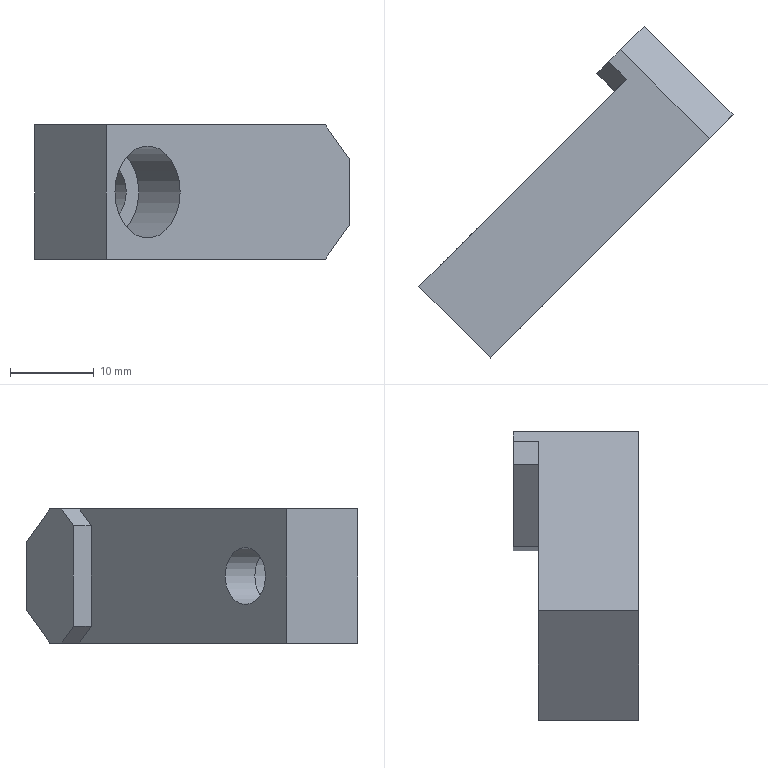Part | STEP file | gslz 2016.10.28-13_id1390_x_t | 1 solid | 15 faces | box 37.477 x 39.598 x 16 mm | volume 7157 mm3 | plane 13 | cylinder 2 | commonest cylinder face diameters 6.8 x1 11 x1
STEP:
#1=CARTESIAN_POINT('',(0.,0.,0.));
#2=DIRECTION('',(0.,0.,1.));
#3=DIRECTION('',(1.,0.,0.));
#4=AXIS2_PLACEMENT_3D('',#1,#2,#3);
#5=CARTESIAN_POINT('',(610.287,162.938,-7.623));
#6=VERTEX_POINT('',#5);
#7=CARTESIAN_POINT('',(584.124,136.775,-7.623));
#8=VERTEX_POINT('',#7);
#9=CARTESIAN_POINT('',(612.408,165.059,-7.623));
#10=DIRECTION('',(-0.7071,-0.7071,0.));
#11=VECTOR('',#10,1.);
#12=LINE('',#9,#11);
#13=CARTESIAN_POINT('',(610.994,166.473,-7.623));
#14=DIRECTION('',(0.,0.,-1.));
#15=DIRECTION('',(0.6428,-0.766,0.));
#16=AXIS2_PLACEMENT_3D('',#13,#14,#15);
#17=PLANE('',#16);
#18=CARTESIAN_POINT('',(1.992,-0.1743));
#19=DIRECTION('',(0.08716,0.9962));
#20=VECTOR('',#19,1.);
#21=LINE('',#18,#20);
#22=(GEOMETRIC_REPRESENTATION_CONTEXT(2)PARAMETRIC_REPRESENTATION_CONTEXT()REPRESENTATION_CONTEXT('',''));
#23=DEFINITIONAL_REPRESENTATION('',(#21),#22);
#24=PCURVE('',#17,#23);
#25=CARTESIAN_POINT('',(612.408,165.059,-37.123));
#26=DIRECTION('',(0.7071,-0.7071,0.));
#27=DIRECTION('',(-0.7071,-0.7071,0.));
#28=AXIS2_PLACEMENT_3D('',#25,#26,#27);
#29=PLANE('',#28);
#30=CARTESIAN_POINT('',(0.,-29.5));
#31=DIRECTION('',(1.,0.));
#32=VECTOR('',#31,1.);
#33=LINE('',#30,#32);
#34=(GEOMETRIC_REPRESENTATION_CONTEXT(2)PARAMETRIC_REPRESENTATION_CONTEXT()REPRESENTATION_CONTEXT('',''));
#35=DEFINITIONAL_REPRESENTATION('',(#33),#34);
#36=PCURVE('',#29,#35);
#37=SURFACE_CURVE('',#12,(#24,#36),.PCURVE_S1.);
#38=EDGE_CURVE('',#6,#8,#37,.T.);
#39=ORIENTED_EDGE('',*,*,#38,.F.);
#40=CARTESIAN_POINT('',(599.68,173.544,-7.623));
#41=VERTEX_POINT('',#40);
#42=CARTESIAN_POINT('',(599.68,173.544,-7.623));
#43=DIRECTION('',(-0.7071,0.7071,0.));
#44=VECTOR('',#43,1.);
#45=LINE('',#42,#44);
#46=CARTESIAN_POINT('',(-12.689,4.122));
#47=DIRECTION('',(-0.9962,0.08716));
#48=VECTOR('',#47,1.);
#49=LINE('',#46,#48);
#50=(GEOMETRIC_REPRESENTATION_CONTEXT(2)PARAMETRIC_REPRESENTATION_CONTEXT()REPRESENTATION_CONTEXT('',''));
#51=DEFINITIONAL_REPRESENTATION('',(#49),#50);
#52=PCURVE('',#17,#51);
#53=CARTESIAN_POINT('',(611.701,167.18,-11.623));
#54=DIRECTION('',(0.5,0.5,0.7071));
#55=DIRECTION('',(-0.7071,0.7071,0.));
#56=AXIS2_PLACEMENT_3D('',#53,#54,#55);
#57=PLANE('',#56);
#58=CARTESIAN_POINT('',(13.,5.657));
#59=DIRECTION('',(1.,0.));
#60=VECTOR('',#59,1.);
#61=LINE('',#58,#60);
#62=(GEOMETRIC_REPRESENTATION_CONTEXT(2)PARAMETRIC_REPRESENTATION_CONTEXT()REPRESENTATION_CONTEXT('',''));
#63=DEFINITIONAL_REPRESENTATION('',(#61),#62);
#64=PCURVE('',#57,#63);
#65=SURFACE_CURVE('',#45,(#52,#64),.PCURVE_S1.);
#66=EDGE_CURVE('',#6,#41,#65,.T.);
#67=ORIENTED_EDGE('',*,*,#66,.T.);
#68=CARTESIAN_POINT('',(598.266,172.13,-7.623));
#69=VERTEX_POINT('',#68);
#70=CARTESIAN_POINT('',(601.802,175.666,-7.623));
#71=DIRECTION('',(-0.7071,-0.7071,0.));
#72=VECTOR('',#71,1.);
#73=LINE('',#70,#72);
#74=CARTESIAN_POINT('',(-12.951,1.133));
#75=DIRECTION('',(0.08716,0.9962));
#76=VECTOR('',#75,1.);
#77=LINE('',#74,#76);
#78=(GEOMETRIC_REPRESENTATION_CONTEXT(2)PARAMETRIC_REPRESENTATION_CONTEXT()REPRESENTATION_CONTEXT('',''));
#79=DEFINITIONAL_REPRESENTATION('',(#77),#78);
#80=PCURVE('',#17,#79);
#81=CARTESIAN_POINT('',(598.266,172.13,-37.123));
#82=DIRECTION('',(0.7071,-0.7071,0.));
#83=DIRECTION('',(-0.7071,-0.7071,0.));
#84=AXIS2_PLACEMENT_3D('',#81,#82,#83);
#85=PLANE('',#84);
#86=CARTESIAN_POINT('',(-5.,-29.5));
#87=DIRECTION('',(1.,0.));
#88=VECTOR('',#87,1.);
#89=LINE('',#86,#88);
#90=(GEOMETRIC_REPRESENTATION_CONTEXT(2)PARAMETRIC_REPRESENTATION_CONTEXT()REPRESENTATION_CONTEXT('',''));
#91=DEFINITIONAL_REPRESENTATION('',(#89),#90);
#92=PCURVE('',#85,#91);
#93=SURFACE_CURVE('',#73,(#80,#92),.PCURVE_S1.);
#94=EDGE_CURVE('',#41,#69,#93,.T.);
#95=ORIENTED_EDGE('',*,*,#94,.T.);
#96=CARTESIAN_POINT('',(600.387,170.009,-7.623));
#97=VERTEX_POINT('',#96);
#98=CARTESIAN_POINT('',(607.458,162.938,-7.623));
#99=DIRECTION('',(0.7071,-0.7071,0.));
#100=VECTOR('',#99,1.);
#101=LINE('',#98,#100);
#102=CARTESIAN_POINT('',(0.4358,4.981));
#103=DIRECTION('',(0.9962,-0.08716));
#104=VECTOR('',#103,1.);
#105=LINE('',#102,#104);
#106=(GEOMETRIC_REPRESENTATION_CONTEXT(2)PARAMETRIC_REPRESENTATION_CONTEXT()REPRESENTATION_CONTEXT('',''));
#107=DEFINITIONAL_REPRESENTATION('',(#105),#106);
#108=PCURVE('',#17,#107);
#109=CARTESIAN_POINT('',(608.873,164.352,-5.623));
#110=DIRECTION('',(0.5,0.5,-0.7071));
#111=DIRECTION('',(-0.7071,0.7071,0.));
#112=AXIS2_PLACEMENT_3D('',#109,#110,#111);
#113=PLANE('',#112);
#114=CARTESIAN_POINT('',(0.,-2.828));
#115=DIRECTION('',(-1.,0.));
#116=VECTOR('',#115,1.);
#117=LINE('',#114,#116);
#118=(GEOMETRIC_REPRESENTATION_CONTEXT(2)PARAMETRIC_REPRESENTATION_CONTEXT()REPRESENTATION_CONTEXT('',''));
#119=DEFINITIONAL_REPRESENTATION('',(#117),#118);
#120=PCURVE('',#113,#119);
#121=SURFACE_CURVE('',#101,(#108,#120),.PCURVE_S1.);
#122=EDGE_CURVE('',#69,#97,#121,.T.);
#123=ORIENTED_EDGE('',*,*,#122,.T.);
#124=CARTESIAN_POINT('',(575.639,145.26,-7.623));
#125=VERTEX_POINT('',#124);
#126=CARTESIAN_POINT('',(603.923,173.544,-7.623));
#127=DIRECTION('',(-0.7071,-0.7071,0.));
#128=VECTOR('',#127,1.);
#129=LINE('',#126,#128);
#130=CARTESIAN_POINT('',(-9.962,0.8716));
#131=DIRECTION('',(0.08716,0.9962));
#132=VECTOR('',#131,1.);
#133=LINE('',#130,#132);
#134=(GEOMETRIC_REPRESENTATION_CONTEXT(2)PARAMETRIC_REPRESENTATION_CONTEXT()REPRESENTATION_CONTEXT('',''));
#135=DEFINITIONAL_REPRESENTATION('',(#133),#134);
#136=PCURVE('',#17,#135);
#137=CARTESIAN_POINT('',(603.923,173.544,-37.123));
#138=DIRECTION('',(0.7071,-0.7071,0.));
#139=DIRECTION('',(-0.7071,-0.7071,0.));
#140=AXIS2_PLACEMENT_3D('',#137,#138,#139);
#141=PLANE('',#140);
#142=CARTESIAN_POINT('',(0.,-29.5));
#143=DIRECTION('',(1.,0.));
#144=VECTOR('',#143,1.);
#145=LINE('',#142,#144);
#146=(GEOMETRIC_REPRESENTATION_CONTEXT(2)PARAMETRIC_REPRESENTATION_CONTEXT()REPRESENTATION_CONTEXT('',''));
#147=DEFINITIONAL_REPRESENTATION('',(#145),#146);
#148=PCURVE('',#141,#147);
#149=SURFACE_CURVE('',#129,(#136,#148),.PCURVE_S1.);
#150=EDGE_CURVE('',#97,#125,#149,.T.);
#151=ORIENTED_EDGE('',*,*,#150,.T.);
#152=CARTESIAN_POINT('',(582.71,138.189,-7.623));
#153=DIRECTION('',(0.7071,-0.7071,0.));
#154=VECTOR('',#153,1.);
#155=LINE('',#152,#154);
#156=CARTESIAN_POINT('',(3.486,39.848));
#157=DIRECTION('',(0.9962,-0.08716));
#158=VECTOR('',#157,1.);
#159=LINE('',#156,#158);
#160=(GEOMETRIC_REPRESENTATION_CONTEXT(2)PARAMETRIC_REPRESENTATION_CONTEXT()REPRESENTATION_CONTEXT('',''));
#161=DEFINITIONAL_REPRESENTATION('',(#159),#160);
#162=PCURVE('',#17,#161);
#163=CARTESIAN_POINT('',(582.71,138.189,-37.123));
#164=DIRECTION('',(-0.7071,-0.7071,0.));
#165=DIRECTION('',(0.7071,-0.7071,0.));
#166=AXIS2_PLACEMENT_3D('',#163,#164,#165);
#167=PLANE('',#166);
#168=CARTESIAN_POINT('',(0.,29.5));
#169=DIRECTION('',(1.,0.));
#170=VECTOR('',#169,1.);
#171=LINE('',#168,#170);
#172=(GEOMETRIC_REPRESENTATION_CONTEXT(2)PARAMETRIC_REPRESENTATION_CONTEXT()REPRESENTATION_CONTEXT('',''));
#173=DEFINITIONAL_REPRESENTATION('',(#171),#172);
#174=PCURVE('',#167,#173);
#175=SURFACE_CURVE('',#155,(#162,#174),.PCURVE_S1.);
#176=EDGE_CURVE('',#125,#8,#175,.T.);
#177=ORIENTED_EDGE('',*,*,#176,.T.);
#178=EDGE_LOOP('',(#39,#67,#95,#123,#151,#177));
#179=FACE_BOUND('',#178,.T.);
#180=ADVANCED_FACE('',(#179),#17,.F.);
#181=CARTESIAN_POINT('',(613.115,165.766,-19.623));
#182=VERTEX_POINT('',#181);
#183=CARTESIAN_POINT('',(613.115,165.766,-11.623));
#184=VERTEX_POINT('',#183);
#185=CARTESIAN_POINT('',(613.115,165.766,-37.123));
#186=DIRECTION('',(0.,0.,1.));
#187=VECTOR('',#186,1.);
#188=LINE('',#185,#187);
#189=CARTESIAN_POINT('',(611.701,167.18,-37.123));
#190=DIRECTION('',(0.7071,0.7071,0.));
#191=DIRECTION('',(0.7071,-0.7071,0.));
#192=AXIS2_PLACEMENT_3D('',#189,#190,#191);
#193=PLANE('',#192);
#194=CARTESIAN_POINT('',(2.,0.));
#195=DIRECTION('',(0.,-1.));
#196=VECTOR('',#195,1.);
#197=LINE('',#194,#196);
#198=(GEOMETRIC_REPRESENTATION_CONTEXT(2)PARAMETRIC_REPRESENTATION_CONTEXT()REPRESENTATION_CONTEXT('',''));
#199=DEFINITIONAL_REPRESENTATION('',(#197),#198);
#200=PCURVE('',#193,#199);
#201=CARTESIAN_POINT('',(-1.,0.));
#202=DIRECTION('',(0.,-1.));
#203=VECTOR('',#202,1.);
#204=LINE('',#201,#203);
#205=(GEOMETRIC_REPRESENTATION_CONTEXT(2)PARAMETRIC_REPRESENTATION_CONTEXT()REPRESENTATION_CONTEXT('',''));
#206=DEFINITIONAL_REPRESENTATION('',(#204),#205);
#207=PCURVE('',#29,#206);
#208=SURFACE_CURVE('',#188,(#200,#207),.PCURVE_S1.);
#209=EDGE_CURVE('',#182,#184,#208,.T.);
#210=ORIENTED_EDGE('',*,*,#209,.F.);
#211=CARTESIAN_POINT('',(602.509,176.373,-19.623));
#212=VERTEX_POINT('',#211);
#213=CARTESIAN_POINT('',(611.701,167.18,-19.623));
#214=DIRECTION('',(-0.7071,0.7071,0.));
#215=VECTOR('',#214,1.);
#216=LINE('',#213,#215);
#217=CARTESIAN_POINT('',(0.,-17.5));
#218=DIRECTION('',(-1.,0.));
#219=VECTOR('',#218,1.);
#220=LINE('',#217,#219);
#221=(GEOMETRIC_REPRESENTATION_CONTEXT(2)PARAMETRIC_REPRESENTATION_CONTEXT()REPRESENTATION_CONTEXT('',''));
#222=DEFINITIONAL_REPRESENTATION('',(#220),#221);
#223=PCURVE('',#193,#222);
#224=CARTESIAN_POINT('',(608.873,164.352,-23.623));
#225=DIRECTION('',(-0.5,-0.5,0.7071));
#226=DIRECTION('',(0.7071,-0.7071,0.));
#227=AXIS2_PLACEMENT_3D('',#224,#225,#226);
#228=PLANE('',#227);
#229=CARTESIAN_POINT('',(0.,5.657));
#230=DIRECTION('',(-1.,0.));
#231=VECTOR('',#230,1.);
#232=LINE('',#229,#231);
#233=(GEOMETRIC_REPRESENTATION_CONTEXT(2)PARAMETRIC_REPRESENTATION_CONTEXT()REPRESENTATION_CONTEXT('',''));
#234=DEFINITIONAL_REPRESENTATION('',(#232),#233);
#235=PCURVE('',#228,#234);
#236=SURFACE_CURVE('',#216,(#223,#235),.PCURVE_S1.);
#237=EDGE_CURVE('',#182,#212,#236,.T.);
#238=ORIENTED_EDGE('',*,*,#237,.T.);
#239=CARTESIAN_POINT('',(602.509,176.373,-11.623));
#240=VERTEX_POINT('',#239);
#241=CARTESIAN_POINT('',(602.509,176.373,-37.123));
#242=DIRECTION('',(0.,0.,-1.));
#243=VECTOR('',#242,1.);
#244=LINE('',#241,#243);
#245=CARTESIAN_POINT('',(-13.,0.));
#246=DIRECTION('',(0.,1.));
#247=VECTOR('',#246,1.);
#248=LINE('',#245,#247);
#249=(GEOMETRIC_REPRESENTATION_CONTEXT(2)PARAMETRIC_REPRESENTATION_CONTEXT()REPRESENTATION_CONTEXT('',''));
#250=DEFINITIONAL_REPRESENTATION('',(#248),#249);
#251=PCURVE('',#193,#250);
#252=CARTESIAN_POINT('',(-6.,0.));
#253=DIRECTION('',(0.,1.));
#254=VECTOR('',#253,1.);
#255=LINE('',#252,#254);
#256=(GEOMETRIC_REPRESENTATION_CONTEXT(2)PARAMETRIC_REPRESENTATION_CONTEXT()REPRESENTATION_CONTEXT('',''));
#257=DEFINITIONAL_REPRESENTATION('',(#255),#256);
#258=PCURVE('',#85,#257);
#259=SURFACE_CURVE('',#244,(#251,#258),.PCURVE_S1.);
#260=EDGE_CURVE('',#240,#212,#259,.T.);
#261=ORIENTED_EDGE('',*,*,#260,.F.);
#262=CARTESIAN_POINT('',(613.115,165.766,-11.623));
#263=DIRECTION('',(0.7071,-0.7071,0.));
#264=VECTOR('',#263,1.);
#265=LINE('',#262,#264);
#266=CARTESIAN_POINT('',(2.,-25.5));
#267=DIRECTION('',(1.,0.));
#268=VECTOR('',#267,1.);
#269=LINE('',#266,#268);
#270=(GEOMETRIC_REPRESENTATION_CONTEXT(2)PARAMETRIC_REPRESENTATION_CONTEXT()REPRESENTATION_CONTEXT('',''));
#271=DEFINITIONAL_REPRESENTATION('',(#269),#270);
#272=PCURVE('',#193,#271);
#273=CARTESIAN_POINT('',(-2.,0.));
#274=DIRECTION('',(-1.,0.));
#275=VECTOR('',#274,1.);
#276=LINE('',#273,#275);
#277=(GEOMETRIC_REPRESENTATION_CONTEXT(2)PARAMETRIC_REPRESENTATION_CONTEXT()REPRESENTATION_CONTEXT('',''));
#278=DEFINITIONAL_REPRESENTATION('',(#276),#277);
#279=PCURVE('',#57,#278);
#280=SURFACE_CURVE('',#265,(#272,#279),.PCURVE_S1.);
#281=EDGE_CURVE('',#240,#184,#280,.T.);
#282=ORIENTED_EDGE('',*,*,#281,.T.);
#283=EDGE_LOOP('',(#210,#238,#261,#282));
#284=FACE_BOUND('',#283,.T.);
#285=ADVANCED_FACE('',(#284),#193,.T.);
#286=CARTESIAN_POINT('',(610.287,162.938,-23.623));
#287=VERTEX_POINT('',#286);
#288=CARTESIAN_POINT('',(584.124,136.775,-23.623));
#289=VERTEX_POINT('',#288);
#290=CARTESIAN_POINT('',(612.408,165.059,-23.623));
#291=DIRECTION('',(-0.7071,-0.7071,0.));
#292=VECTOR('',#291,1.);
#293=LINE('',#290,#292);
#294=CARTESIAN_POINT('',(0.,-13.5));
#295=DIRECTION('',(1.,0.));
#296=VECTOR('',#295,1.);
#297=LINE('',#294,#296);
#298=(GEOMETRIC_REPRESENTATION_CONTEXT(2)PARAMETRIC_REPRESENTATION_CONTEXT()REPRESENTATION_CONTEXT('',''));
#299=DEFINITIONAL_REPRESENTATION('',(#297),#298);
#300=PCURVE('',#29,#299);
#301=CARTESIAN_POINT('',(610.994,166.473,-23.623));
#302=DIRECTION('',(0.,0.,-1.));
#303=DIRECTION('',(0.6428,-0.766,0.));
#304=AXIS2_PLACEMENT_3D('',#301,#302,#303);
#305=PLANE('',#304);
#306=CARTESIAN_POINT('',(1.992,-0.1743));
#307=DIRECTION('',(0.08716,0.9962));
#308=VECTOR('',#307,1.);
#309=LINE('',#306,#308);
#310=(GEOMETRIC_REPRESENTATION_CONTEXT(2)PARAMETRIC_REPRESENTATION_CONTEXT()REPRESENTATION_CONTEXT('',''));
#311=DEFINITIONAL_REPRESENTATION('',(#309),#310);
#312=PCURVE('',#305,#311);
#313=SURFACE_CURVE('',#293,(#300,#312),.PCURVE_S1.);
#314=EDGE_CURVE('',#287,#289,#313,.T.);
#315=ORIENTED_EDGE('',*,*,#314,.F.);
#316=CARTESIAN_POINT('',(606.575,159.225,-28.873));
#317=DIRECTION('',(0.5,0.5,0.7071));
#318=VECTOR('',#317,1.);
#319=LINE('',#316,#318);
#320=CARTESIAN_POINT('',(8.25,-8.25));
#321=DIRECTION('',(-0.7071,-0.7071));
#322=VECTOR('',#321,1.);
#323=LINE('',#320,#322);
#324=(GEOMETRIC_REPRESENTATION_CONTEXT(2)PARAMETRIC_REPRESENTATION_CONTEXT()REPRESENTATION_CONTEXT('',''));
#325=DEFINITIONAL_REPRESENTATION('',(#323),#324);
#326=PCURVE('',#29,#325);
#327=CARTESIAN_POINT('',(2.,-7.425));
#328=DIRECTION('',(0.,1.));
#329=VECTOR('',#328,1.);
#330=LINE('',#327,#329);
#331=(GEOMETRIC_REPRESENTATION_CONTEXT(2)PARAMETRIC_REPRESENTATION_CONTEXT()REPRESENTATION_CONTEXT('',''));
#332=DEFINITIONAL_REPRESENTATION('',(#330),#331);
#333=PCURVE('',#228,#332);
#334=SURFACE_CURVE('',#319,(#326,#333),.PCURVE_S1.);
#335=EDGE_CURVE('',#287,#182,#334,.T.);
#336=ORIENTED_EDGE('',*,*,#335,.T.);
#337=ORIENTED_EDGE('',*,*,#209,.T.);
#338=CARTESIAN_POINT('',(621.777,174.428,-23.873));
#339=DIRECTION('',(-0.5,-0.5,0.7071));
#340=VECTOR('',#339,1.);
#341=LINE('',#338,#340);
#342=CARTESIAN_POINT('',(-13.25,-13.25));
#343=DIRECTION('',(0.7071,-0.7071));
#344=VECTOR('',#343,1.);
#345=LINE('',#342,#344);
#346=(GEOMETRIC_REPRESENTATION_CONTEXT(2)PARAMETRIC_REPRESENTATION_CONTEXT()REPRESENTATION_CONTEXT('',''));
#347=DEFINITIONAL_REPRESENTATION('',(#345),#346);
#348=PCURVE('',#29,#347);
#349=CARTESIAN_POINT('',(-2.,-17.324));
#350=DIRECTION('',(0.,1.));
#351=VECTOR('',#350,1.);
#352=LINE('',#349,#351);
#353=(GEOMETRIC_REPRESENTATION_CONTEXT(2)PARAMETRIC_REPRESENTATION_CONTEXT()REPRESENTATION_CONTEXT('',''));
#354=DEFINITIONAL_REPRESENTATION('',(#352),#353);
#355=PCURVE('',#57,#354);
#356=SURFACE_CURVE('',#341,(#348,#355),.PCURVE_S1.);
#357=EDGE_CURVE('',#184,#6,#356,.T.);
#358=ORIENTED_EDGE('',*,*,#357,.T.);
#359=ORIENTED_EDGE('',*,*,#38,.T.);
#360=CARTESIAN_POINT('',(584.124,136.775,-37.123));
#361=DIRECTION('',(0.,0.,-1.));
#362=VECTOR('',#361,1.);
#363=LINE('',#360,#362);
#364=CARTESIAN_POINT('',(40.,0.));
#365=DIRECTION('',(0.,1.));
#366=VECTOR('',#365,1.);
#367=LINE('',#364,#366);
#368=(GEOMETRIC_REPRESENTATION_CONTEXT(2)PARAMETRIC_REPRESENTATION_CONTEXT()REPRESENTATION_CONTEXT('',''));
#369=DEFINITIONAL_REPRESENTATION('',(#367),#368);
#370=PCURVE('',#29,#369);
#371=CARTESIAN_POINT('',(2.,0.));
#372=DIRECTION('',(0.,-1.));
#373=VECTOR('',#372,1.);
#374=LINE('',#371,#373);
#375=(GEOMETRIC_REPRESENTATION_CONTEXT(2)PARAMETRIC_REPRESENTATION_CONTEXT()REPRESENTATION_CONTEXT('',''));
#376=DEFINITIONAL_REPRESENTATION('',(#374),#375);
#377=PCURVE('',#167,#376);
#378=SURFACE_CURVE('',#363,(#370,#377),.PCURVE_S1.);
#379=EDGE_CURVE('',#8,#289,#378,.T.);
#380=ORIENTED_EDGE('',*,*,#379,.T.);
#381=EDGE_LOOP('',(#315,#336,#337,#358,#359,#380));
#382=FACE_BOUND('',#381,.T.);
#383=CARTESIAN_POINT('',(592.963,145.614,-15.623));
#384=VERTEX_POINT('',#383);
#385=CARTESIAN_POINT('',(589.074,141.724,-15.623));
#386=DIRECTION('',(0.7071,-0.7071,0.));
#387=DIRECTION('',(0.7071,0.7071,0.));
#388=AXIS2_PLACEMENT_3D('',#385,#386,#387);
#389=CIRCLE('',#388,5.5);
#390=CARTESIAN_POINT('',(33.,-21.5));
#391=DIRECTION('',(-1.,0.));
#392=AXIS2_PLACEMENT_2D('',#390,#391);
#393=CIRCLE('',#392,5.5);
#394=(GEOMETRIC_REPRESENTATION_CONTEXT(2)PARAMETRIC_REPRESENTATION_CONTEXT()REPRESENTATION_CONTEXT('',''));
#395=DEFINITIONAL_REPRESENTATION('',(#393),#394);
#396=PCURVE('',#29,#395);
#397=CARTESIAN_POINT('',(593.316,137.482,-15.623));
#398=DIRECTION('',(-0.7071,0.7071,0.));
#399=DIRECTION('',(0.7071,0.7071,0.));
#400=AXIS2_PLACEMENT_3D('',#397,#398,#399);
#401=CYLINDRICAL_SURFACE('',#400,5.5);
#402=CARTESIAN_POINT('',(6.283,6.));
#403=DIRECTION('',(-1.,0.));
#404=VECTOR('',#403,1.);
#405=LINE('',#402,#404);
#406=(GEOMETRIC_REPRESENTATION_CONTEXT(2)PARAMETRIC_REPRESENTATION_CONTEXT()REPRESENTATION_CONTEXT('',''));
#407=DEFINITIONAL_REPRESENTATION('',(#405),#406);
#408=PCURVE('',#401,#407);
#409=SURFACE_CURVE('',#389,(#396,#408),.PCURVE_S1.);
#410=EDGE_CURVE('',#384,#384,#409,.T.);
#411=ORIENTED_EDGE('',*,*,#410,.F.);
#412=EDGE_LOOP('',(#411));
#413=FACE_BOUND('',#412,.T.);
#414=ADVANCED_FACE('',(#382,#413),#29,.T.);
#415=CARTESIAN_POINT('',(600.387,170.009,-23.623));
#416=VERTEX_POINT('',#415);
#417=CARTESIAN_POINT('',(575.639,145.26,-23.623));
#418=VERTEX_POINT('',#417);
#419=CARTESIAN_POINT('',(603.923,173.544,-23.623));
#420=DIRECTION('',(-0.7071,-0.7071,0.));
#421=VECTOR('',#420,1.);
#422=LINE('',#419,#421);
#423=CARTESIAN_POINT('',(0.,-13.5));
#424=DIRECTION('',(1.,0.));
#425=VECTOR('',#424,1.);
#426=LINE('',#423,#425);
#427=(GEOMETRIC_REPRESENTATION_CONTEXT(2)PARAMETRIC_REPRESENTATION_CONTEXT()REPRESENTATION_CONTEXT('',''));
#428=DEFINITIONAL_REPRESENTATION('',(#426),#427);
#429=PCURVE('',#141,#428);
#430=CARTESIAN_POINT('',(-9.962,0.8716));
#431=DIRECTION('',(0.08716,0.9962));
#432=VECTOR('',#431,1.);
#433=LINE('',#430,#432);
#434=(GEOMETRIC_REPRESENTATION_CONTEXT(2)PARAMETRIC_REPRESENTATION_CONTEXT()REPRESENTATION_CONTEXT('',''));
#435=DEFINITIONAL_REPRESENTATION('',(#433),#434);
#436=PCURVE('',#305,#435);
#437=SURFACE_CURVE('',#422,(#429,#436),.PCURVE_S1.);
#438=EDGE_CURVE('',#416,#418,#437,.T.);
#439=ORIENTED_EDGE('',*,*,#438,.T.);
#440=CARTESIAN_POINT('',(575.639,145.26,-37.123));
#441=DIRECTION('',(0.,0.,-1.));
#442=VECTOR('',#441,1.);
#443=LINE('',#440,#442);
#444=CARTESIAN_POINT('',(40.,0.));
#445=DIRECTION('',(0.,1.));
#446=VECTOR('',#445,1.);
#447=LINE('',#444,#446);
#448=(GEOMETRIC_REPRESENTATION_CONTEXT(2)PARAMETRIC_REPRESENTATION_CONTEXT()REPRESENTATION_CONTEXT('',''));
#449=DEFINITIONAL_REPRESENTATION('',(#447),#448);
#450=PCURVE('',#141,#449);
#451=CARTESIAN_POINT('',(-10.,0.));
#452=DIRECTION('',(0.,-1.));
#453=VECTOR('',#452,1.);
#454=LINE('',#451,#453);
#455=(GEOMETRIC_REPRESENTATION_CONTEXT(2)PARAMETRIC_REPRESENTATION_CONTEXT()REPRESENTATION_CONTEXT('',''));
#456=DEFINITIONAL_REPRESENTATION('',(#454),#455);
#457=PCURVE('',#167,#456);
#458=SURFACE_CURVE('',#443,(#450,#457),.PCURVE_S1.);
#459=EDGE_CURVE('',#125,#418,#458,.T.);
#460=ORIENTED_EDGE('',*,*,#459,.F.);
#461=ORIENTED_EDGE('',*,*,#150,.F.);
#462=CARTESIAN_POINT('',(598.973,168.594,-9.623));
#463=VERTEX_POINT('',#462);
#464=CARTESIAN_POINT('',(582.886,152.508,-32.373));
#465=DIRECTION('',(-0.5,-0.5,-0.7071));
#466=VECTOR('',#465,1.);
#467=LINE('',#464,#466);
#468=CARTESIAN_POINT('',(29.75,-4.75));
#469=DIRECTION('',(0.7071,0.7071));
#470=VECTOR('',#469,1.);
#471=LINE('',#468,#470);
#472=(GEOMETRIC_REPRESENTATION_CONTEXT(2)PARAMETRIC_REPRESENTATION_CONTEXT()REPRESENTATION_CONTEXT('',''));
#473=DEFINITIONAL_REPRESENTATION('',(#471),#472);
#474=PCURVE('',#141,#473);
#475=CARTESIAN_POINT('',(10.,-37.83));
#476=DIRECTION('',(0.,-1.));
#477=VECTOR('',#476,1.);
#478=LINE('',#475,#477);
#479=(GEOMETRIC_REPRESENTATION_CONTEXT(2)PARAMETRIC_REPRESENTATION_CONTEXT()REPRESENTATION_CONTEXT('',''));
#480=DEFINITIONAL_REPRESENTATION('',(#478),#479);
#481=PCURVE('',#113,#480);
#482=SURFACE_CURVE('',#467,(#474,#481),.PCURVE_S1.);
#483=EDGE_CURVE('',#97,#463,#482,.T.);
#484=ORIENTED_EDGE('',*,*,#483,.T.);
#485=CARTESIAN_POINT('',(598.973,168.594,-21.623));
#486=VERTEX_POINT('',#485);
#487=CARTESIAN_POINT('',(598.973,168.594,-37.123));
#488=DIRECTION('',(0.,0.,1.));
#489=VECTOR('',#488,1.);
#490=LINE('',#487,#489);
#491=CARTESIAN_POINT('',(7.,0.));
#492=DIRECTION('',(0.,-1.));
#493=VECTOR('',#492,1.);
#494=LINE('',#491,#493);
#495=(GEOMETRIC_REPRESENTATION_CONTEXT(2)PARAMETRIC_REPRESENTATION_CONTEXT()REPRESENTATION_CONTEXT('',''));
#496=DEFINITIONAL_REPRESENTATION('',(#494),#495);
#497=PCURVE('',#141,#496);
#498=CARTESIAN_POINT('',(605.337,162.231,-15.623));
#499=DIRECTION('',(0.7071,0.7071,0.));
#500=DIRECTION('',(0.7071,-0.7071,0.));
#501=AXIS2_PLACEMENT_3D('',#498,#499,#500);
#502=PLANE('',#501);
#503=CARTESIAN_POINT('',(-9.,21.5));
#504=DIRECTION('',(0.,-1.));
#505=VECTOR('',#504,1.);
#506=LINE('',#503,#505);
#507=(GEOMETRIC_REPRESENTATION_CONTEXT(2)PARAMETRIC_REPRESENTATION_CONTEXT()REPRESENTATION_CONTEXT('',''));
#508=DEFINITIONAL_REPRESENTATION('',(#506),#507);
#509=PCURVE('',#502,#508);
#510=SURFACE_CURVE('',#490,(#497,#509),.PCURVE_S1.);
#511=EDGE_CURVE('',#486,#463,#510,.T.);
#512=ORIENTED_EDGE('',*,*,#511,.F.);
#513=CARTESIAN_POINT('',(598.089,167.711,-20.373));
#514=DIRECTION('',(0.5,0.5,-0.7071));
#515=VECTOR('',#514,1.);
#516=LINE('',#513,#515);
#517=CARTESIAN_POINT('',(8.25,-16.75));
#518=DIRECTION('',(-0.7071,0.7071));
#519=VECTOR('',#518,1.);
#520=LINE('',#517,#519);
#521=(GEOMETRIC_REPRESENTATION_CONTEXT(2)PARAMETRIC_REPRESENTATION_CONTEXT()REPRESENTATION_CONTEXT('',''));
#522=DEFINITIONAL_REPRESENTATION('',(#520),#521);
#523=PCURVE('',#141,#522);
#524=CARTESIAN_POINT('',(608.873,164.352,-25.623));
#525=DIRECTION('',(-0.5,-0.5,-0.7071));
#526=DIRECTION('',(-0.7071,0.7071,0.));
#527=AXIS2_PLACEMENT_3D('',#524,#525,#526);
#528=PLANE('',#527);
#529=CARTESIAN_POINT('',(10.,-7.425));
#530=DIRECTION('',(0.,1.));
#531=VECTOR('',#530,1.);
#532=LINE('',#529,#531);
#533=(GEOMETRIC_REPRESENTATION_CONTEXT(2)PARAMETRIC_REPRESENTATION_CONTEXT()REPRESENTATION_CONTEXT('',''));
#534=DEFINITIONAL_REPRESENTATION('',(#532),#533);
#535=PCURVE('',#528,#534);
#536=SURFACE_CURVE('',#516,(#523,#535),.PCURVE_S1.);
#537=EDGE_CURVE('',#486,#416,#536,.T.);
#538=ORIENTED_EDGE('',*,*,#537,.T.);
#539=EDGE_LOOP('',(#439,#460,#461,#484,#512,#538));
#540=FACE_BOUND('',#539,.T.);
#541=CARTESIAN_POINT('',(582.993,152.614,-15.623));
#542=VERTEX_POINT('',#541);
#543=CARTESIAN_POINT('',(580.588,150.21,-15.623));
#544=DIRECTION('',(-0.7071,0.7071,0.));
#545=DIRECTION('',(0.7071,0.7071,0.));
#546=AXIS2_PLACEMENT_3D('',#543,#544,#545);
#547=CIRCLE('',#546,3.4);
#548=CARTESIAN_POINT('',(29.6,-21.5));
#549=CARTESIAN_POINT('',(29.6,-15.611));
#550=CARTESIAN_POINT('',(34.7,-18.556));
#551=CARTESIAN_POINT('',(39.8,-21.5));
#552=CARTESIAN_POINT('',(34.7,-24.444));
#553=CARTESIAN_POINT('',(29.6,-27.389));
#554=CARTESIAN_POINT('',(29.6,-21.5));
#555=(BOUNDED_CURVE()B_SPLINE_CURVE(2,(#548,#549,#550,#551,#552,#553,#554),.UNSPECIFIED.,.T.,.F.)B_SPLINE_CURVE_WITH_KNOTS((1,2,2,2,2,1),(-2.094,0.,2.094,4.189,6.283,8.378),.UNSPECIFIED.)CURVE()GEOMETRIC_REPRESENTATION_ITEM()RATIONAL_B_SPLINE_CURVE((1.,0.5,1.,0.5,1.,0.5,1.))REPRESENTATION_ITEM(''));
#556=(GEOMETRIC_REPRESENTATION_CONTEXT(2)PARAMETRIC_REPRESENTATION_CONTEXT()REPRESENTATION_CONTEXT('',''));
#557=DEFINITIONAL_REPRESENTATION('',(#555),#556);
#558=PCURVE('',#141,#557);
#559=CARTESIAN_POINT('',(514.827,215.971,-15.623));
#560=DIRECTION('',(-0.7071,0.7071,0.));
#561=DIRECTION('',(0.7071,0.7071,0.));
#562=AXIS2_PLACEMENT_3D('',#559,#560,#561);
#563=CYLINDRICAL_SURFACE('',#562,3.4);
#564=CARTESIAN_POINT('',(0.,-93.));
#565=DIRECTION('',(1.,0.));
#566=VECTOR('',#565,1.);
#567=LINE('',#564,#566);
#568=(GEOMETRIC_REPRESENTATION_CONTEXT(2)PARAMETRIC_REPRESENTATION_CONTEXT()REPRESENTATION_CONTEXT('',''));
#569=DEFINITIONAL_REPRESENTATION('',(#567),#568);
#570=PCURVE('',#563,#569);
#571=SURFACE_CURVE('',#547,(#558,#570),.PCURVE_S1.);
#572=EDGE_CURVE('',#542,#542,#571,.T.);
#573=ORIENTED_EDGE('',*,*,#572,.F.);
#574=EDGE_LOOP('',(#573));
#575=FACE_BOUND('',#574,.T.);
#576=ADVANCED_FACE('',(#540,#575),#141,.F.);
#577=CARTESIAN_POINT('',(599.68,173.544,-23.623));
#578=VERTEX_POINT('',#577);
#579=CARTESIAN_POINT('',(598.266,172.13,-23.623));
#580=VERTEX_POINT('',#579);
#581=CARTESIAN_POINT('',(601.802,175.666,-23.623));
#582=DIRECTION('',(-0.7071,-0.7071,0.));
#583=VECTOR('',#582,1.);
#584=LINE('',#581,#583);
#585=CARTESIAN_POINT('',(-12.951,1.133));
#586=DIRECTION('',(0.08716,0.9962));
#587=VECTOR('',#586,1.);
#588=LINE('',#585,#587);
#589=(GEOMETRIC_REPRESENTATION_CONTEXT(2)PARAMETRIC_REPRESENTATION_CONTEXT()REPRESENTATION_CONTEXT('',''));
#590=DEFINITIONAL_REPRESENTATION('',(#588),#589);
#591=PCURVE('',#305,#590);
#592=CARTESIAN_POINT('',(-5.,-13.5));
#593=DIRECTION('',(1.,0.));
#594=VECTOR('',#593,1.);
#595=LINE('',#592,#594);
#596=(GEOMETRIC_REPRESENTATION_CONTEXT(2)PARAMETRIC_REPRESENTATION_CONTEXT()REPRESENTATION_CONTEXT('',''));
#597=DEFINITIONAL_REPRESENTATION('',(#595),#596);
#598=PCURVE('',#85,#597);
#599=SURFACE_CURVE('',#584,(#591,#598),.PCURVE_S1.);
#600=EDGE_CURVE('',#578,#580,#599,.T.);
#601=ORIENTED_EDGE('',*,*,#600,.F.);
#602=CARTESIAN_POINT('',(608.873,164.352,-23.623));
#603=DIRECTION('',(0.7071,-0.7071,0.));
#604=VECTOR('',#603,1.);
#605=LINE('',#602,#604);
#606=CARTESIAN_POINT('',(0.2615,2.989));
#607=DIRECTION('',(0.9962,-0.08716));
#608=VECTOR('',#607,1.);
#609=LINE('',#606,#608);
#610=(GEOMETRIC_REPRESENTATION_CONTEXT(2)PARAMETRIC_REPRESENTATION_CONTEXT()REPRESENTATION_CONTEXT('',''));
#611=DEFINITIONAL_REPRESENTATION('',(#609),#610);
#612=PCURVE('',#305,#611);
#613=CARTESIAN_POINT('',(0.,0.));
#614=DIRECTION('',(1.,0.));
#615=VECTOR('',#614,1.);
#616=LINE('',#613,#615);
#617=(GEOMETRIC_REPRESENTATION_CONTEXT(2)PARAMETRIC_REPRESENTATION_CONTEXT()REPRESENTATION_CONTEXT('',''));
#618=DEFINITIONAL_REPRESENTATION('',(#616),#617);
#619=PCURVE('',#228,#618);
#620=SURFACE_CURVE('',#605,(#612,#619),.PCURVE_S1.);
#621=EDGE_CURVE('',#578,#287,#620,.T.);
#622=ORIENTED_EDGE('',*,*,#621,.T.);
#623=ORIENTED_EDGE('',*,*,#314,.T.);
#624=CARTESIAN_POINT('',(582.71,138.189,-23.623));
#625=DIRECTION('',(0.7071,-0.7071,0.));
#626=VECTOR('',#625,1.);
#627=LINE('',#624,#626);
#628=CARTESIAN_POINT('',(3.486,39.848));
#629=DIRECTION('',(0.9962,-0.08716));
#630=VECTOR('',#629,1.);
#631=LINE('',#628,#630);
#632=(GEOMETRIC_REPRESENTATION_CONTEXT(2)PARAMETRIC_REPRESENTATION_CONTEXT()REPRESENTATION_CONTEXT('',''));
#633=DEFINITIONAL_REPRESENTATION('',(#631),#632);
#634=PCURVE('',#305,#633);
#635=CARTESIAN_POINT('',(0.,13.5));
#636=DIRECTION('',(1.,0.));
#637=VECTOR('',#636,1.);
#638=LINE('',#635,#637);
#639=(GEOMETRIC_REPRESENTATION_CONTEXT(2)PARAMETRIC_REPRESENTATION_CONTEXT()REPRESENTATION_CONTEXT('',''));
#640=DEFINITIONAL_REPRESENTATION('',(#638),#639);
#641=PCURVE('',#167,#640);
#642=SURFACE_CURVE('',#627,(#634,#641),.PCURVE_S1.);
#643=EDGE_CURVE('',#418,#289,#642,.T.);
#644=ORIENTED_EDGE('',*,*,#643,.F.);
#645=ORIENTED_EDGE('',*,*,#438,.F.);
#646=CARTESIAN_POINT('',(607.458,162.938,-23.623));
#647=DIRECTION('',(-0.7071,0.7071,0.));
#648=VECTOR('',#647,1.);
#649=LINE('',#646,#648);
#650=CARTESIAN_POINT('',(0.4358,4.981));
#651=DIRECTION('',(-0.9962,0.08716));
#652=VECTOR('',#651,1.);
#653=LINE('',#650,#652);
#654=(GEOMETRIC_REPRESENTATION_CONTEXT(2)PARAMETRIC_REPRESENTATION_CONTEXT()REPRESENTATION_CONTEXT('',''));
#655=DEFINITIONAL_REPRESENTATION('',(#653),#654);
#656=PCURVE('',#305,#655);
#657=CARTESIAN_POINT('',(0.,-2.828));
#658=DIRECTION('',(1.,0.));
#659=VECTOR('',#658,1.);
#660=LINE('',#657,#659);
#661=(GEOMETRIC_REPRESENTATION_CONTEXT(2)PARAMETRIC_REPRESENTATION_CONTEXT()REPRESENTATION_CONTEXT('',''));
#662=DEFINITIONAL_REPRESENTATION('',(#660),#661);
#663=PCURVE('',#528,#662);
#664=SURFACE_CURVE('',#649,(#656,#663),.PCURVE_S1.);
#665=EDGE_CURVE('',#416,#580,#664,.T.);
#666=ORIENTED_EDGE('',*,*,#665,.T.);
#667=EDGE_LOOP('',(#601,#622,#623,#644,#645,#666));
#668=FACE_BOUND('',#667,.T.);
#669=ADVANCED_FACE('',(#668),#305,.T.);
#670=ORIENTED_EDGE('',*,*,#260,.T.);
#671=CARTESIAN_POINT('',(599.68,173.544,-23.623));
#672=DIRECTION('',(-0.5,-0.5,-0.7071));
#673=VECTOR('',#672,1.);
#674=LINE('',#671,#673);
#675=CARTESIAN_POINT('',(-2.,-13.5));
#676=DIRECTION('',(0.7071,0.7071));
#677=VECTOR('',#676,1.);
#678=LINE('',#675,#677);
#679=(GEOMETRIC_REPRESENTATION_CONTEXT(2)PARAMETRIC_REPRESENTATION_CONTEXT()REPRESENTATION_CONTEXT('',''));
#680=DEFINITIONAL_REPRESENTATION('',(#678),#679);
#681=PCURVE('',#85,#680);
#682=CARTESIAN_POINT('',(-13.,0.));
#683=DIRECTION('',(0.,-1.));
#684=VECTOR('',#683,1.);
#685=LINE('',#682,#684);
#686=(GEOMETRIC_REPRESENTATION_CONTEXT(2)PARAMETRIC_REPRESENTATION_CONTEXT()REPRESENTATION_CONTEXT('',''));
#687=DEFINITIONAL_REPRESENTATION('',(#685),#686);
#688=PCURVE('',#228,#687);
#689=SURFACE_CURVE('',#674,(#681,#688),.PCURVE_S1.);
#690=EDGE_CURVE('',#212,#578,#689,.T.);
#691=ORIENTED_EDGE('',*,*,#690,.T.);
#692=ORIENTED_EDGE('',*,*,#600,.T.);
#693=CARTESIAN_POINT('',(596.852,170.716,-21.623));
#694=VERTEX_POINT('',#693);
#695=CARTESIAN_POINT('',(599.68,173.544,-25.623));
#696=DIRECTION('',(-0.5,-0.5,0.7071));
#697=VECTOR('',#696,1.);
#698=LINE('',#695,#697);
#699=CARTESIAN_POINT('',(-2.,-11.5));
#700=DIRECTION('',(0.7071,-0.7071));
#701=VECTOR('',#700,1.);
#702=LINE('',#699,#701);
#703=(GEOMETRIC_REPRESENTATION_CONTEXT(2)PARAMETRIC_REPRESENTATION_CONTEXT()REPRESENTATION_CONTEXT('',''));
#704=DEFINITIONAL_REPRESENTATION('',(#702),#703);
#705=PCURVE('',#85,#704);
#706=CARTESIAN_POINT('',(13.,0.));
#707=DIRECTION('',(0.,-1.));
#708=VECTOR('',#707,1.);
#709=LINE('',#706,#708);
#710=(GEOMETRIC_REPRESENTATION_CONTEXT(2)PARAMETRIC_REPRESENTATION_CONTEXT()REPRESENTATION_CONTEXT('',''));
#711=DEFINITIONAL_REPRESENTATION('',(#709),#710);
#712=PCURVE('',#528,#711);
#713=SURFACE_CURVE('',#698,(#705,#712),.PCURVE_S1.);
#714=EDGE_CURVE('',#580,#694,#713,.T.);
#715=ORIENTED_EDGE('',*,*,#714,.T.);
#716=CARTESIAN_POINT('',(596.852,170.716,-9.623));
#717=VERTEX_POINT('',#716);
#718=CARTESIAN_POINT('',(596.852,170.716,-37.123));
#719=DIRECTION('',(0.,0.,-1.));
#720=VECTOR('',#719,1.);
#721=LINE('',#718,#720);
#722=CARTESIAN_POINT('',(2.,0.));
#723=DIRECTION('',(0.,1.));
#724=VECTOR('',#723,1.);
#725=LINE('',#722,#724);
#726=(GEOMETRIC_REPRESENTATION_CONTEXT(2)PARAMETRIC_REPRESENTATION_CONTEXT()REPRESENTATION_CONTEXT('',''));
#727=DEFINITIONAL_REPRESENTATION('',(#725),#726);
#728=PCURVE('',#85,#727);
#729=CARTESIAN_POINT('',(-12.,21.5));
#730=DIRECTION('',(0.,1.));
#731=VECTOR('',#730,1.);
#732=LINE('',#729,#731);
#733=(GEOMETRIC_REPRESENTATION_CONTEXT(2)PARAMETRIC_REPRESENTATION_CONTEXT()REPRESENTATION_CONTEXT('',''));
#734=DEFINITIONAL_REPRESENTATION('',(#732),#733);
#735=PCURVE('',#502,#734);
#736=SURFACE_CURVE('',#721,(#728,#735),.PCURVE_S1.);
#737=EDGE_CURVE('',#717,#694,#736,.T.);
#738=ORIENTED_EDGE('',*,*,#737,.F.);
#739=CARTESIAN_POINT('',(599.68,173.544,-5.623));
#740=DIRECTION('',(0.5,0.5,0.7071));
#741=VECTOR('',#740,1.);
#742=LINE('',#739,#741);
#743=CARTESIAN_POINT('',(-2.,-31.5));
#744=DIRECTION('',(-0.7071,-0.7071));
#745=VECTOR('',#744,1.);
#746=LINE('',#743,#745);
#747=(GEOMETRIC_REPRESENTATION_CONTEXT(2)PARAMETRIC_REPRESENTATION_CONTEXT()REPRESENTATION_CONTEXT('',''));
#748=DEFINITIONAL_REPRESENTATION('',(#746),#747);
#749=PCURVE('',#85,#748);
#750=CARTESIAN_POINT('',(13.,0.));
#751=DIRECTION('',(0.,1.));
#752=VECTOR('',#751,1.);
#753=LINE('',#750,#752);
#754=(GEOMETRIC_REPRESENTATION_CONTEXT(2)PARAMETRIC_REPRESENTATION_CONTEXT()REPRESENTATION_CONTEXT('',''));
#755=DEFINITIONAL_REPRESENTATION('',(#753),#754);
#756=PCURVE('',#113,#755);
#757=SURFACE_CURVE('',#742,(#749,#756),.PCURVE_S1.);
#758=EDGE_CURVE('',#717,#69,#757,.T.);
#759=ORIENTED_EDGE('',*,*,#758,.T.);
#760=ORIENTED_EDGE('',*,*,#94,.F.);
#761=CARTESIAN_POINT('',(602.509,176.373,-11.623));
#762=DIRECTION('',(0.5,0.5,-0.7071));
#763=VECTOR('',#762,1.);
#764=LINE('',#761,#763);
#765=CARTESIAN_POINT('',(-6.,-25.5));
#766=DIRECTION('',(-0.7071,0.7071));
#767=VECTOR('',#766,1.);
#768=LINE('',#765,#767);
#769=(GEOMETRIC_REPRESENTATION_CONTEXT(2)PARAMETRIC_REPRESENTATION_CONTEXT()REPRESENTATION_CONTEXT('',''));
#770=DEFINITIONAL_REPRESENTATION('',(#768),#769);
#771=PCURVE('',#85,#770);
#772=CARTESIAN_POINT('',(13.,0.));
#773=DIRECTION('',(0.,-1.));
#774=VECTOR('',#773,1.);
#775=LINE('',#772,#774);
#776=(GEOMETRIC_REPRESENTATION_CONTEXT(2)PARAMETRIC_REPRESENTATION_CONTEXT()REPRESENTATION_CONTEXT('',''));
#777=DEFINITIONAL_REPRESENTATION('',(#775),#776);
#778=PCURVE('',#57,#777);
#779=SURFACE_CURVE('',#764,(#771,#778),.PCURVE_S1.);
#780=EDGE_CURVE('',#41,#240,#779,.T.);
#781=ORIENTED_EDGE('',*,*,#780,.T.);
#782=EDGE_LOOP('',(#670,#691,#692,#715,#738,#759,#760,#781));
#783=FACE_BOUND('',#782,.T.);
#784=ADVANCED_FACE('',(#783),#85,.F.);
#785=ORIENTED_EDGE('',*,*,#737,.T.);
#786=CARTESIAN_POINT('',(598.973,168.594,-21.623));
#787=DIRECTION('',(0.7071,-0.7071,0.));
#788=VECTOR('',#787,1.);
#789=LINE('',#786,#788);
#790=CARTESIAN_POINT('',(-9.,6.));
#791=DIRECTION('',(1.,0.));
#792=VECTOR('',#791,1.);
#793=LINE('',#790,#792);
#794=(GEOMETRIC_REPRESENTATION_CONTEXT(2)PARAMETRIC_REPRESENTATION_CONTEXT()REPRESENTATION_CONTEXT('',''));
#795=DEFINITIONAL_REPRESENTATION('',(#793),#794);
#796=PCURVE('',#502,#795);
#797=CARTESIAN_POINT('',(10.,-5.657));
#798=DIRECTION('',(-1.,0.));
#799=VECTOR('',#798,1.);
#800=LINE('',#797,#799);
#801=(GEOMETRIC_REPRESENTATION_CONTEXT(2)PARAMETRIC_REPRESENTATION_CONTEXT()REPRESENTATION_CONTEXT('',''));
#802=DEFINITIONAL_REPRESENTATION('',(#800),#801);
#803=PCURVE('',#528,#802);
#804=SURFACE_CURVE('',#789,(#796,#803),.PCURVE_S1.);
#805=EDGE_CURVE('',#694,#486,#804,.T.);
#806=ORIENTED_EDGE('',*,*,#805,.T.);
#807=ORIENTED_EDGE('',*,*,#511,.T.);
#808=CARTESIAN_POINT('',(605.337,162.231,-9.623));
#809=DIRECTION('',(-0.7071,0.7071,0.));
#810=VECTOR('',#809,1.);
#811=LINE('',#808,#810);
#812=CARTESIAN_POINT('',(0.,-6.));
#813=DIRECTION('',(-1.,0.));
#814=VECTOR('',#813,1.);
#815=LINE('',#812,#814);
#816=(GEOMETRIC_REPRESENTATION_CONTEXT(2)PARAMETRIC_REPRESENTATION_CONTEXT()REPRESENTATION_CONTEXT('',''));
#817=DEFINITIONAL_REPRESENTATION('',(#815),#816);
#818=PCURVE('',#502,#817);
#819=CARTESIAN_POINT('',(1.,-5.657));
#820=DIRECTION('',(1.,0.));
#821=VECTOR('',#820,1.);
#822=LINE('',#819,#821);
#823=(GEOMETRIC_REPRESENTATION_CONTEXT(2)PARAMETRIC_REPRESENTATION_CONTEXT()REPRESENTATION_CONTEXT('',''));
#824=DEFINITIONAL_REPRESENTATION('',(#822),#823);
#825=PCURVE('',#113,#824);
#826=SURFACE_CURVE('',#811,(#818,#825),.PCURVE_S1.);
#827=EDGE_CURVE('',#463,#717,#826,.T.);
#828=ORIENTED_EDGE('',*,*,#827,.T.);
#829=EDGE_LOOP('',(#785,#806,#807,#828));
#830=FACE_BOUND('',#829,.T.);
#831=ADVANCED_FACE('',(#830),#502,.F.);
#832=ORIENTED_EDGE('',*,*,#379,.F.);
#833=ORIENTED_EDGE('',*,*,#176,.F.);
#834=ORIENTED_EDGE('',*,*,#459,.T.);
#835=ORIENTED_EDGE('',*,*,#643,.T.);
#836=EDGE_LOOP('',(#832,#833,#834,#835));
#837=FACE_BOUND('',#836,.T.);
#838=ADVANCED_FACE('',(#837),#167,.T.);
#839=CARTESIAN_POINT('',(581.72,144.27,-15.623));
#840=VERTEX_POINT('',#839);
#841=CARTESIAN_POINT('',(586.528,149.078,-15.623));
#842=VERTEX_POINT('',#841);
#843=CARTESIAN_POINT('',(584.124,146.674,-15.623));
#844=DIRECTION('',(-0.7071,0.7071,0.));
#845=DIRECTION('',(-0.7071,-0.7071,0.));
#846=AXIS2_PLACEMENT_3D('',#843,#844,#845);
#847=CIRCLE('',#846,3.4);
#848=CARTESIAN_POINT('',(3.142,-98.));
#849=DIRECTION('',(1.,0.));
#850=VECTOR('',#849,1.);
#851=LINE('',#848,#850);
#852=(GEOMETRIC_REPRESENTATION_CONTEXT(2)PARAMETRIC_REPRESENTATION_CONTEXT()REPRESENTATION_CONTEXT('',''));
#853=DEFINITIONAL_REPRESENTATION('',(#851),#852);
#854=PCURVE('',#563,#853);
#855=CARTESIAN_POINT('',(584.831,147.381,-15.623));
#856=DIRECTION('',(-0.7071,0.7071,0.));
#857=DIRECTION('',(0.7071,0.7071,0.));
#858=AXIS2_PLACEMENT_3D('',#855,#856,#857);
#859=PLANE('',#858);
#860=CARTESIAN_POINT('',(-1.,0.));
#861=DIRECTION('',(-1.,0.));
#862=AXIS2_PLACEMENT_2D('',#860,#861);
#863=CIRCLE('',#862,3.4);
#864=(GEOMETRIC_REPRESENTATION_CONTEXT(2)PARAMETRIC_REPRESENTATION_CONTEXT()REPRESENTATION_CONTEXT('',''));
#865=DEFINITIONAL_REPRESENTATION('',(#863),#864);
#866=PCURVE('',#859,#865);
#867=SURFACE_CURVE('',#847,(#854,#866),.PCURVE_S1.);
#868=EDGE_CURVE('',#840,#842,#867,.T.);
#869=ORIENTED_EDGE('',*,*,#868,.T.);
#870=CARTESIAN_POINT('',(586.528,149.078,-15.623));
#871=CARTESIAN_POINT('',(582.993,152.614,-15.623));
#872=B_SPLINE_CURVE_WITH_KNOTS('',1,(#870,#871),.UNSPECIFIED.,.F.,.F.,(2,2),(-98.,-93.),.PIECEWISE_BEZIER_KNOTS.);
#873=CARTESIAN_POINT('',(6.283,0.));
#874=DIRECTION('',(0.,1.));
#875=VECTOR('',#874,1.);
#876=LINE('',#873,#875);
#877=(GEOMETRIC_REPRESENTATION_CONTEXT(2)PARAMETRIC_REPRESENTATION_CONTEXT()REPRESENTATION_CONTEXT('',''));
#878=DEFINITIONAL_REPRESENTATION('',(#876),#877);
#879=PCURVE('',#563,#878);
#880=CARTESIAN_POINT('',(0.,0.));
#881=DIRECTION('',(0.,1.));
#882=VECTOR('',#881,1.);
#883=LINE('',#880,#882);
#884=(GEOMETRIC_REPRESENTATION_CONTEXT(2)PARAMETRIC_REPRESENTATION_CONTEXT()REPRESENTATION_CONTEXT('',''));
#885=DEFINITIONAL_REPRESENTATION('',(#883),#884);
#886=PCURVE('',#563,#885);
#887=SEAM_CURVE('',#872,(#879,#886),.PCURVE_S1.);
#888=EDGE_CURVE('',#842,#542,#887,.T.);
#889=ORIENTED_EDGE('',*,*,#888,.T.);
#890=ORIENTED_EDGE('',*,*,#572,.F.);
#891=ORIENTED_EDGE('',*,*,#888,.F.);
#892=CARTESIAN_POINT('',(584.124,146.674,-15.623));
#893=DIRECTION('',(-0.7071,0.7071,0.));
#894=DIRECTION('',(-0.7071,-0.7071,0.));
#895=AXIS2_PLACEMENT_3D('',#892,#893,#894);
#896=CIRCLE('',#895,3.4);
#897=CARTESIAN_POINT('',(-3.142,-98.));
#898=DIRECTION('',(1.,0.));
#899=VECTOR('',#898,1.);
#900=LINE('',#897,#899);
#901=(GEOMETRIC_REPRESENTATION_CONTEXT(2)PARAMETRIC_REPRESENTATION_CONTEXT()REPRESENTATION_CONTEXT('',''));
#902=DEFINITIONAL_REPRESENTATION('',(#900),#901);
#903=PCURVE('',#563,#902);
#904=CARTESIAN_POINT('',(-1.,0.));
#905=DIRECTION('',(-1.,0.));
#906=AXIS2_PLACEMENT_2D('',#904,#905);
#907=CIRCLE('',#906,3.4);
#908=(GEOMETRIC_REPRESENTATION_CONTEXT(2)PARAMETRIC_REPRESENTATION_CONTEXT()REPRESENTATION_CONTEXT('',''));
#909=DEFINITIONAL_REPRESENTATION('',(#907),#908);
#910=PCURVE('',#859,#909);
#911=SURFACE_CURVE('',#896,(#903,#910),.PCURVE_S1.);
#912=EDGE_CURVE('',#842,#840,#911,.T.);
#913=ORIENTED_EDGE('',*,*,#912,.T.);
#914=EDGE_LOOP('',(#869,#889,#890,#891,#913));
#915=FACE_BOUND('',#914,.F.);
#916=ADVANCED_FACE('',(#915),#563,.F.);
#917=ORIENTED_EDGE('',*,*,#868,.T.);
#918=ORIENTED_EDGE('',*,*,#912,.T.);
#919=EDGE_LOOP('',(#917,#918));
#920=FACE_BOUND('',#919,.T.);
#921=CARTESIAN_POINT('',(580.235,142.785,-15.623));
#922=VERTEX_POINT('',#921);
#923=CARTESIAN_POINT('',(588.013,150.563,-15.623));
#924=VERTEX_POINT('',#923);
#925=CARTESIAN_POINT('',(584.124,146.674,-15.623));
#926=DIRECTION('',(-0.7071,0.7071,0.));
#927=DIRECTION('',(-0.7071,-0.7071,0.));
#928=AXIS2_PLACEMENT_3D('',#925,#926,#927);
#929=CIRCLE('',#928,5.5);
#930=CARTESIAN_POINT('',(-1.,0.));
#931=DIRECTION('',(-1.,0.));
#932=AXIS2_PLACEMENT_2D('',#930,#931);
#933=CIRCLE('',#932,5.5);
#934=(GEOMETRIC_REPRESENTATION_CONTEXT(2)PARAMETRIC_REPRESENTATION_CONTEXT()REPRESENTATION_CONTEXT('',''));
#935=DEFINITIONAL_REPRESENTATION('',(#933),#934);
#936=PCURVE('',#859,#935);
#937=CARTESIAN_POINT('',(3.142,13.));
#938=DIRECTION('',(1.,0.));
#939=VECTOR('',#938,1.);
#940=LINE('',#937,#939);
#941=(GEOMETRIC_REPRESENTATION_CONTEXT(2)PARAMETRIC_REPRESENTATION_CONTEXT()REPRESENTATION_CONTEXT('',''));
#942=DEFINITIONAL_REPRESENTATION('',(#940),#941);
#943=PCURVE('',#401,#942);
#944=SURFACE_CURVE('',#929,(#936,#943),.PCURVE_S1.);
#945=EDGE_CURVE('',#922,#924,#944,.T.);
#946=ORIENTED_EDGE('',*,*,#945,.F.);
#947=CARTESIAN_POINT('',(584.124,146.674,-15.623));
#948=DIRECTION('',(-0.7071,0.7071,0.));
#949=DIRECTION('',(-0.7071,-0.7071,0.));
#950=AXIS2_PLACEMENT_3D('',#947,#948,#949);
#951=CIRCLE('',#950,5.5);
#952=CARTESIAN_POINT('',(-1.,0.));
#953=DIRECTION('',(-1.,0.));
#954=AXIS2_PLACEMENT_2D('',#952,#953);
#955=CIRCLE('',#954,5.5);
#956=(GEOMETRIC_REPRESENTATION_CONTEXT(2)PARAMETRIC_REPRESENTATION_CONTEXT()REPRESENTATION_CONTEXT('',''));
#957=DEFINITIONAL_REPRESENTATION('',(#955),#956);
#958=PCURVE('',#859,#957);
#959=CARTESIAN_POINT('',(-3.142,13.));
#960=DIRECTION('',(1.,0.));
#961=VECTOR('',#960,1.);
#962=LINE('',#959,#961);
#963=(GEOMETRIC_REPRESENTATION_CONTEXT(2)PARAMETRIC_REPRESENTATION_CONTEXT()REPRESENTATION_CONTEXT('',''));
#964=DEFINITIONAL_REPRESENTATION('',(#962),#963);
#965=PCURVE('',#401,#964);
#966=SURFACE_CURVE('',#951,(#958,#965),.PCURVE_S1.);
#967=EDGE_CURVE('',#924,#922,#966,.T.);
#968=ORIENTED_EDGE('',*,*,#967,.F.);
#969=EDGE_LOOP('',(#946,#968));
#970=FACE_BOUND('',#969,.T.);
#971=ADVANCED_FACE('',(#920,#970),#859,.F.);
#972=ORIENTED_EDGE('',*,*,#967,.F.);
#973=CARTESIAN_POINT('',(592.963,145.614,-15.623));
#974=CARTESIAN_POINT('',(588.013,150.563,-15.623));
#975=B_SPLINE_CURVE_WITH_KNOTS('',1,(#973,#974),.UNSPECIFIED.,.F.,.F.,(2,2),(6.,13.),.PIECEWISE_BEZIER_KNOTS.);
#976=CARTESIAN_POINT('',(0.,0.));
#977=DIRECTION('',(0.,1.));
#978=VECTOR('',#977,1.);
#979=LINE('',#976,#978);
#980=(GEOMETRIC_REPRESENTATION_CONTEXT(2)PARAMETRIC_REPRESENTATION_CONTEXT()REPRESENTATION_CONTEXT('',''));
#981=DEFINITIONAL_REPRESENTATION('',(#979),#980);
#982=PCURVE('',#401,#981);
#983=CARTESIAN_POINT('',(6.283,0.));
#984=DIRECTION('',(0.,1.));
#985=VECTOR('',#984,1.);
#986=LINE('',#983,#985);
#987=(GEOMETRIC_REPRESENTATION_CONTEXT(2)PARAMETRIC_REPRESENTATION_CONTEXT()REPRESENTATION_CONTEXT('',''));
#988=DEFINITIONAL_REPRESENTATION('',(#986),#987);
#989=PCURVE('',#401,#988);
#990=SEAM_CURVE('',#975,(#982,#989),.PCURVE_S1.);
#991=EDGE_CURVE('',#384,#924,#990,.T.);
#992=ORIENTED_EDGE('',*,*,#991,.F.);
#993=ORIENTED_EDGE('',*,*,#410,.F.);
#994=ORIENTED_EDGE('',*,*,#991,.T.);
#995=ORIENTED_EDGE('',*,*,#945,.F.);
#996=EDGE_LOOP('',(#972,#992,#993,#994,#995));
#997=FACE_BOUND('',#996,.F.);
#998=ADVANCED_FACE('',(#997),#401,.F.);
#999=ORIENTED_EDGE('',*,*,#537,.F.);
#1000=ORIENTED_EDGE('',*,*,#805,.F.);
#1001=ORIENTED_EDGE('',*,*,#714,.F.);
#1002=ORIENTED_EDGE('',*,*,#665,.F.);
#1003=EDGE_LOOP('',(#999,#1000,#1001,#1002));
#1004=FACE_BOUND('',#1003,.T.);
#1005=ADVANCED_FACE('',(#1004),#528,.T.);
#1006=ORIENTED_EDGE('',*,*,#758,.F.);
#1007=ORIENTED_EDGE('',*,*,#827,.F.);
#1008=ORIENTED_EDGE('',*,*,#483,.F.);
#1009=ORIENTED_EDGE('',*,*,#122,.F.);
#1010=EDGE_LOOP('',(#1006,#1007,#1008,#1009));
#1011=FACE_BOUND('',#1010,.T.);
#1012=ADVANCED_FACE('',(#1011),#113,.F.);
#1013=ORIENTED_EDGE('',*,*,#690,.F.);
#1014=ORIENTED_EDGE('',*,*,#237,.F.);
#1015=ORIENTED_EDGE('',*,*,#335,.F.);
#1016=ORIENTED_EDGE('',*,*,#621,.F.);
#1017=EDGE_LOOP('',(#1013,#1014,#1015,#1016));
#1018=FACE_BOUND('',#1017,.T.);
#1019=ADVANCED_FACE('',(#1018),#228,.F.);
#1020=ORIENTED_EDGE('',*,*,#780,.F.);
#1021=ORIENTED_EDGE('',*,*,#66,.F.);
#1022=ORIENTED_EDGE('',*,*,#357,.F.);
#1023=ORIENTED_EDGE('',*,*,#281,.F.);
#1024=EDGE_LOOP('',(#1020,#1021,#1022,#1023));
#1025=FACE_BOUND('',#1024,.T.);
#1026=ADVANCED_FACE('',(#1025),#57,.T.);
#1027=CLOSED_SHELL('',(#180,#285,#414,#576,#669,#784,#831,#838,#916,#971,#998,#1005,#1012,#1019,#1026));
#1028=MANIFOLD_SOLID_BREP('',#1027);
#1029=(LENGTH_UNIT()NAMED_UNIT(*)SI_UNIT(.MILLI.,.METRE.));
#1030=UNCERTAINTY_MEASURE_WITH_UNIT(LENGTH_MEASURE(0.000001),#1029,'','');
#1031=(NAMED_UNIT(*)PLANE_ANGLE_UNIT()SI_UNIT($,.RADIAN.));
#1032=(NAMED_UNIT(*)SI_UNIT($,.STERADIAN.)SOLID_ANGLE_UNIT());
#1033=(GEOMETRIC_REPRESENTATION_CONTEXT(3)GLOBAL_UNCERTAINTY_ASSIGNED_CONTEXT((#1030))GLOBAL_UNIT_ASSIGNED_CONTEXT((#1029,#1031,#1032))REPRESENTATION_CONTEXT('',''));
#1034=ADVANCED_BREP_SHAPE_REPRESENTATION('',(#4,#1028),#1033);